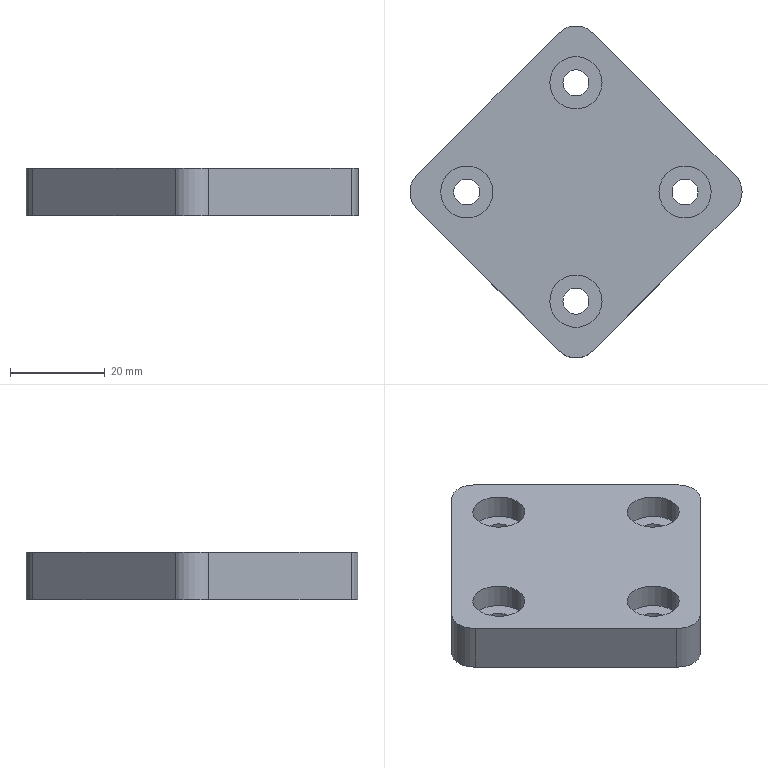Part | SolidWorks | features BaseBody 1 | 1 solid | 31 faces | box 70 x 70 x 10 mm | volume 24895 mm3 | cylinder 21 | plane 10 | commonest cylinder face diameters 5.5 x8 11 x8 10 x5
STEP:
#1=CARTESIAN_POINT('',(-699.595,684.746,545.732));
#2=VERTEX_POINT('',#1);
#3=CARTESIAN_POINT('',(-698.131,681.211,545.732));
#4=VERTEX_POINT('',#3);
#5=CARTESIAN_POINT('',(-703.131,681.211,545.732));
#6=DIRECTION('',(0.,0.,-1.));
#7=DIRECTION('',(0.7071,0.7071,0.));
#8=AXIS2_PLACEMENT_3D('',#5,#6,#7);
#9=CIRCLE('',#8,5.);
#10=EDGE_CURVE('',#2,#4,#9,.T.);
#11=ORIENTED_EDGE('',*,*,#10,.T.);
#12=CARTESIAN_POINT('',(-698.131,681.211,535.732));
#13=VERTEX_POINT('',#12);
#14=CARTESIAN_POINT('',(-698.131,681.211,558.768));
#15=DIRECTION('',(0.,0.,-1.));
#16=VECTOR('',#15,1000.);
#17=LINE('',#14,#16);
#18=EDGE_CURVE('',#4,#13,#17,.T.);
#19=ORIENTED_EDGE('',*,*,#18,.T.);
#20=CARTESIAN_POINT('',(-699.595,684.746,535.732));
#21=VERTEX_POINT('',#20);
#22=CARTESIAN_POINT('',(-703.131,681.211,535.732));
#23=DIRECTION('',(0.,0.,1.));
#24=DIRECTION('',(0.7071,-0.7071,0.));
#25=AXIS2_PLACEMENT_3D('',#22,#23,#24);
#26=CIRCLE('',#25,5.);
#27=EDGE_CURVE('',#13,#21,#26,.T.);
#28=ORIENTED_EDGE('',*,*,#27,.T.);
#29=CARTESIAN_POINT('',(-699.595,684.746,545.732));
#30=DIRECTION('',(0.,0.,-1.));
#31=VECTOR('',#30,1000.);
#32=LINE('',#29,#31);
#33=EDGE_CURVE('',#2,#21,#32,.T.);
#34=ORIENTED_EDGE('',*,*,#33,.F.);
#35=EDGE_LOOP('',(#11,#19,#28,#34));
#36=FACE_OUTER_BOUND('',#35,.T.);
#37=CARTESIAN_POINT('',(-703.131,681.211,558.768));
#38=DIRECTION('',(0.,0.,-1.));
#39=DIRECTION('',(1.,0.,0.));
#40=AXIS2_PLACEMENT_3D('',#37,#38,#39);
#41=CYLINDRICAL_SURFACE('',#40,5.);
#42=ADVANCED_FACE('',(#36),#41,.T.);
#43=CARTESIAN_POINT('',(-729.595,714.746,535.732));
#44=VERTEX_POINT('',#43);
#45=CARTESIAN_POINT('',(-736.666,714.746,535.732));
#46=VERTEX_POINT('',#45);
#47=CARTESIAN_POINT('',(-733.131,711.211,535.732));
#48=DIRECTION('',(0.,0.,1.));
#49=DIRECTION('',(0.7071,0.7071,0.));
#50=AXIS2_PLACEMENT_3D('',#47,#48,#49);
#51=CIRCLE('',#50,5.);
#52=EDGE_CURVE('',#44,#46,#51,.T.);
#53=ORIENTED_EDGE('',*,*,#52,.F.);
#54=CARTESIAN_POINT('',(-699.595,684.746,535.732));
#55=DIRECTION('',(-0.7071,0.7071,0.));
#56=VECTOR('',#55,1000.);
#57=LINE('',#54,#56);
#58=EDGE_CURVE('',#21,#44,#57,.T.);
#59=ORIENTED_EDGE('',*,*,#58,.F.);
#60=ORIENTED_EDGE('',*,*,#27,.F.);
#61=CARTESIAN_POINT('',(-699.595,677.675,535.732));
#62=VERTEX_POINT('',#61);
#63=CARTESIAN_POINT('',(-703.131,681.211,535.732));
#64=DIRECTION('',(0.,0.,1.));
#65=DIRECTION('',(0.7071,-0.7071,0.));
#66=AXIS2_PLACEMENT_3D('',#63,#64,#65);
#67=CIRCLE('',#66,5.);
#68=EDGE_CURVE('',#62,#13,#67,.T.);
#69=ORIENTED_EDGE('',*,*,#68,.F.);
#70=CARTESIAN_POINT('',(-729.595,647.675,535.732));
#71=VERTEX_POINT('',#70);
#72=CARTESIAN_POINT('',(-729.595,647.675,535.732));
#73=DIRECTION('',(0.7071,0.7071,0.));
#74=VECTOR('',#73,1000.);
#75=LINE('',#72,#74);
#76=EDGE_CURVE('',#71,#62,#75,.T.);
#77=ORIENTED_EDGE('',*,*,#76,.F.);
#78=CARTESIAN_POINT('',(-736.666,647.675,535.732));
#79=VERTEX_POINT('',#78);
#80=CARTESIAN_POINT('',(-733.131,651.211,535.732));
#81=DIRECTION('',(0.,0.,1.));
#82=DIRECTION('',(-0.7071,-0.7071,0.));
#83=AXIS2_PLACEMENT_3D('',#80,#81,#82);
#84=CIRCLE('',#83,5.);
#85=EDGE_CURVE('',#79,#71,#84,.T.);
#86=ORIENTED_EDGE('',*,*,#85,.F.);
#87=CARTESIAN_POINT('',(-766.666,677.675,535.732));
#88=VERTEX_POINT('',#87);
#89=CARTESIAN_POINT('',(-766.666,677.675,535.732));
#90=DIRECTION('',(0.7071,-0.7071,0.));
#91=VECTOR('',#90,1000.);
#92=LINE('',#89,#91);
#93=EDGE_CURVE('',#88,#79,#92,.T.);
#94=ORIENTED_EDGE('',*,*,#93,.F.);
#95=CARTESIAN_POINT('',(-766.666,684.746,535.732));
#96=VERTEX_POINT('',#95);
#97=CARTESIAN_POINT('',(-763.131,681.211,535.732));
#98=DIRECTION('',(0.,0.,1.));
#99=DIRECTION('',(-0.7071,0.7071,0.));
#100=AXIS2_PLACEMENT_3D('',#97,#98,#99);
#101=CIRCLE('',#100,5.);
#102=EDGE_CURVE('',#96,#88,#101,.T.);
#103=ORIENTED_EDGE('',*,*,#102,.F.);
#104=CARTESIAN_POINT('',(-736.666,714.746,535.732));
#105=DIRECTION('',(-0.7071,-0.7071,0.));
#106=VECTOR('',#105,1000.);
#107=LINE('',#104,#106);
#108=EDGE_CURVE('',#46,#96,#107,.T.);
#109=ORIENTED_EDGE('',*,*,#108,.F.);
#110=EDGE_LOOP('',(#53,#59,#60,#69,#77,#86,#94,#103,#109));
#111=FACE_OUTER_BOUND('',#110,.T.);
#112=CARTESIAN_POINT('',(-758.881,681.211,535.732));
#113=VERTEX_POINT('',#112);
#114=CARTESIAN_POINT('',(-753.381,681.211,535.732));
#115=VERTEX_POINT('',#114);
#116=CARTESIAN_POINT('',(-756.131,681.211,535.732));
#117=DIRECTION('',(0.,0.,-1.));
#118=DIRECTION('',(-1.,0.,0.));
#119=AXIS2_PLACEMENT_3D('',#116,#117,#118);
#120=CIRCLE('',#119,2.75);
#121=EDGE_CURVE('',#113,#115,#120,.T.);
#122=ORIENTED_EDGE('',*,*,#121,.F.);
#123=CARTESIAN_POINT('',(-756.131,681.211,535.732));
#124=DIRECTION('',(0.,0.,-1.));
#125=DIRECTION('',(1.,0.,0.));
#126=AXIS2_PLACEMENT_3D('',#123,#124,#125);
#127=CIRCLE('',#126,2.75);
#128=EDGE_CURVE('',#115,#113,#127,.T.);
#129=ORIENTED_EDGE('',*,*,#128,.F.);
#130=EDGE_LOOP('',(#122,#129));
#131=FACE_BOUND('',#130,.T.);
#132=CARTESIAN_POINT('',(-712.881,681.211,535.732));
#133=VERTEX_POINT('',#132);
#134=CARTESIAN_POINT('',(-707.381,681.211,535.732));
#135=VERTEX_POINT('',#134);
#136=CARTESIAN_POINT('',(-710.131,681.211,535.732));
#137=DIRECTION('',(0.,0.,-1.));
#138=DIRECTION('',(-1.,0.,0.));
#139=AXIS2_PLACEMENT_3D('',#136,#137,#138);
#140=CIRCLE('',#139,2.75);
#141=EDGE_CURVE('',#133,#135,#140,.T.);
#142=ORIENTED_EDGE('',*,*,#141,.F.);
#143=CARTESIAN_POINT('',(-710.131,681.211,535.732));
#144=DIRECTION('',(0.,0.,-1.));
#145=DIRECTION('',(1.,0.,0.));
#146=AXIS2_PLACEMENT_3D('',#143,#144,#145);
#147=CIRCLE('',#146,2.75);
#148=EDGE_CURVE('',#135,#133,#147,.T.);
#149=ORIENTED_EDGE('',*,*,#148,.F.);
#150=EDGE_LOOP('',(#142,#149));
#151=FACE_BOUND('',#150,.T.);
#152=CARTESIAN_POINT('',(-735.881,658.211,535.732));
#153=VERTEX_POINT('',#152);
#154=CARTESIAN_POINT('',(-730.381,658.211,535.732));
#155=VERTEX_POINT('',#154);
#156=CARTESIAN_POINT('',(-733.131,658.211,535.732));
#157=DIRECTION('',(0.,0.,-1.));
#158=DIRECTION('',(-1.,0.,0.));
#159=AXIS2_PLACEMENT_3D('',#156,#157,#158);
#160=CIRCLE('',#159,2.75);
#161=EDGE_CURVE('',#153,#155,#160,.T.);
#162=ORIENTED_EDGE('',*,*,#161,.F.);
#163=CARTESIAN_POINT('',(-733.131,658.211,535.732));
#164=DIRECTION('',(0.,0.,-1.));
#165=DIRECTION('',(1.,0.,0.));
#166=AXIS2_PLACEMENT_3D('',#163,#164,#165);
#167=CIRCLE('',#166,2.75);
#168=EDGE_CURVE('',#155,#153,#167,.T.);
#169=ORIENTED_EDGE('',*,*,#168,.F.);
#170=EDGE_LOOP('',(#162,#169));
#171=FACE_BOUND('',#170,.T.);
#172=CARTESIAN_POINT('',(-735.881,704.211,535.732));
#173=VERTEX_POINT('',#172);
#174=CARTESIAN_POINT('',(-730.381,704.211,535.732));
#175=VERTEX_POINT('',#174);
#176=CARTESIAN_POINT('',(-733.131,704.211,535.732));
#177=DIRECTION('',(0.,0.,-1.));
#178=DIRECTION('',(-1.,0.,0.));
#179=AXIS2_PLACEMENT_3D('',#176,#177,#178);
#180=CIRCLE('',#179,2.75);
#181=EDGE_CURVE('',#173,#175,#180,.T.);
#182=ORIENTED_EDGE('',*,*,#181,.F.);
#183=CARTESIAN_POINT('',(-733.131,704.211,535.732));
#184=DIRECTION('',(0.,0.,-1.));
#185=DIRECTION('',(1.,0.,0.));
#186=AXIS2_PLACEMENT_3D('',#183,#184,#185);
#187=CIRCLE('',#186,2.75);
#188=EDGE_CURVE('',#175,#173,#187,.T.);
#189=ORIENTED_EDGE('',*,*,#188,.F.);
#190=EDGE_LOOP('',(#182,#189));
#191=FACE_BOUND('',#190,.T.);
#192=CARTESIAN_POINT('',(0.,0.,535.732));
#193=DIRECTION('',(0.,0.,1.));
#194=DIRECTION('',(-1.,0.,0.));
#195=AXIS2_PLACEMENT_3D('',#192,#193,#194);
#196=PLANE('',#195);
#197=ADVANCED_FACE('',(#111,#131,#151,#171,#191),#196,.F.);
#198=CARTESIAN_POINT('',(-736.666,714.746,545.732));
#199=VERTEX_POINT('',#198);
#200=CARTESIAN_POINT('',(-736.666,714.746,545.732));
#201=DIRECTION('',(0.,0.,-1.));
#202=VECTOR('',#201,1000.);
#203=LINE('',#200,#202);
#204=EDGE_CURVE('',#199,#46,#203,.T.);
#205=ORIENTED_EDGE('',*,*,#204,.T.);
#206=ORIENTED_EDGE('',*,*,#108,.T.);
#207=CARTESIAN_POINT('',(-766.666,684.746,545.732));
#208=VERTEX_POINT('',#207);
#209=CARTESIAN_POINT('',(-766.666,684.746,535.732));
#210=DIRECTION('',(0.,0.,1.));
#211=VECTOR('',#210,1000.);
#212=LINE('',#209,#211);
#213=EDGE_CURVE('',#96,#208,#212,.T.);
#214=ORIENTED_EDGE('',*,*,#213,.T.);
#215=CARTESIAN_POINT('',(-766.666,684.746,545.732));
#216=DIRECTION('',(0.7071,0.7071,0.));
#217=VECTOR('',#216,1000.);
#218=LINE('',#215,#217);
#219=EDGE_CURVE('',#208,#199,#218,.T.);
#220=ORIENTED_EDGE('',*,*,#219,.T.);
#221=EDGE_LOOP('',(#205,#206,#214,#220));
#222=FACE_OUTER_BOUND('',#221,.T.);
#223=CARTESIAN_POINT('',(-733.131,718.282,535.732));
#224=DIRECTION('',(-0.7071,0.7071,0.));
#225=DIRECTION('',(0.7071,0.7071,0.));
#226=AXIS2_PLACEMENT_3D('',#223,#224,#225);
#227=PLANE('',#226);
#228=ADVANCED_FACE('',(#222),#227,.T.);
#229=CARTESIAN_POINT('',(-729.595,647.675,545.732));
#230=VERTEX_POINT('',#229);
#231=CARTESIAN_POINT('',(-736.666,647.675,545.732));
#232=VERTEX_POINT('',#231);
#233=CARTESIAN_POINT('',(-733.131,651.211,545.732));
#234=DIRECTION('',(0.,0.,-1.));
#235=DIRECTION('',(0.7071,-0.7071,0.));
#236=AXIS2_PLACEMENT_3D('',#233,#234,#235);
#237=CIRCLE('',#236,5.);
#238=EDGE_CURVE('',#230,#232,#237,.T.);
#239=ORIENTED_EDGE('',*,*,#238,.F.);
#240=CARTESIAN_POINT('',(-699.595,677.675,545.732));
#241=VERTEX_POINT('',#240);
#242=CARTESIAN_POINT('',(-699.595,677.675,545.732));
#243=DIRECTION('',(-0.7071,-0.7071,0.));
#244=VECTOR('',#243,1000.);
#245=LINE('',#242,#244);
#246=EDGE_CURVE('',#241,#230,#245,.T.);
#247=ORIENTED_EDGE('',*,*,#246,.F.);
#248=CARTESIAN_POINT('',(-703.131,681.211,545.732));
#249=DIRECTION('',(0.,0.,-1.));
#250=DIRECTION('',(0.7071,0.7071,0.));
#251=AXIS2_PLACEMENT_3D('',#248,#249,#250);
#252=CIRCLE('',#251,5.);
#253=EDGE_CURVE('',#4,#241,#252,.T.);
#254=ORIENTED_EDGE('',*,*,#253,.F.);
#255=ORIENTED_EDGE('',*,*,#10,.F.);
#256=CARTESIAN_POINT('',(-729.595,714.746,545.732));
#257=VERTEX_POINT('',#256);
#258=CARTESIAN_POINT('',(-729.595,714.746,545.732));
#259=DIRECTION('',(0.7071,-0.7071,0.));
#260=VECTOR('',#259,1000.);
#261=LINE('',#258,#260);
#262=EDGE_CURVE('',#257,#2,#261,.T.);
#263=ORIENTED_EDGE('',*,*,#262,.F.);
#264=CARTESIAN_POINT('',(-733.131,711.211,545.732));
#265=DIRECTION('',(0.,0.,-1.));
#266=DIRECTION('',(-0.7071,0.7071,0.));
#267=AXIS2_PLACEMENT_3D('',#264,#265,#266);
#268=CIRCLE('',#267,5.);
#269=EDGE_CURVE('',#199,#257,#268,.T.);
#270=ORIENTED_EDGE('',*,*,#269,.F.);
#271=ORIENTED_EDGE('',*,*,#219,.F.);
#272=CARTESIAN_POINT('',(-766.666,677.675,545.732));
#273=VERTEX_POINT('',#272);
#274=CARTESIAN_POINT('',(-763.131,681.211,545.732));
#275=DIRECTION('',(0.,0.,-1.));
#276=DIRECTION('',(-0.7071,-0.7071,0.));
#277=AXIS2_PLACEMENT_3D('',#274,#275,#276);
#278=CIRCLE('',#277,5.);
#279=EDGE_CURVE('',#273,#208,#278,.T.);
#280=ORIENTED_EDGE('',*,*,#279,.F.);
#281=CARTESIAN_POINT('',(-736.666,647.675,545.732));
#282=DIRECTION('',(-0.7071,0.7071,0.));
#283=VECTOR('',#282,1000.);
#284=LINE('',#281,#283);
#285=EDGE_CURVE('',#232,#273,#284,.T.);
#286=ORIENTED_EDGE('',*,*,#285,.F.);
#287=EDGE_LOOP('',(#239,#247,#254,#255,#263,#270,#271,#280,#286));
#288=FACE_OUTER_BOUND('',#287,.T.);
#289=CARTESIAN_POINT('',(-727.631,704.211,545.732));
#290=VERTEX_POINT('',#289);
#291=CARTESIAN_POINT('',(-738.631,704.211,545.732));
#292=VERTEX_POINT('',#291);
#293=CARTESIAN_POINT('',(-733.131,704.211,545.732));
#294=DIRECTION('',(0.,0.,1.));
#295=DIRECTION('',(1.,0.,0.));
#296=AXIS2_PLACEMENT_3D('',#293,#294,#295);
#297=CIRCLE('',#296,5.5);
#298=EDGE_CURVE('',#290,#292,#297,.T.);
#299=ORIENTED_EDGE('',*,*,#298,.F.);
#300=CARTESIAN_POINT('',(-733.131,704.211,545.732));
#301=DIRECTION('',(0.,0.,1.));
#302=DIRECTION('',(-1.,0.,0.));
#303=AXIS2_PLACEMENT_3D('',#300,#301,#302);
#304=CIRCLE('',#303,5.5);
#305=EDGE_CURVE('',#292,#290,#304,.T.);
#306=ORIENTED_EDGE('',*,*,#305,.F.);
#307=EDGE_LOOP('',(#299,#306));
#308=FACE_BOUND('',#307,.T.);
#309=CARTESIAN_POINT('',(-704.631,681.211,545.732));
#310=VERTEX_POINT('',#309);
#311=CARTESIAN_POINT('',(-715.631,681.211,545.732));
#312=VERTEX_POINT('',#311);
#313=CARTESIAN_POINT('',(-710.131,681.211,545.732));
#314=DIRECTION('',(0.,0.,1.));
#315=DIRECTION('',(1.,0.,0.));
#316=AXIS2_PLACEMENT_3D('',#313,#314,#315);
#317=CIRCLE('',#316,5.5);
#318=EDGE_CURVE('',#310,#312,#317,.T.);
#319=ORIENTED_EDGE('',*,*,#318,.F.);
#320=CARTESIAN_POINT('',(-710.131,681.211,545.732));
#321=DIRECTION('',(0.,0.,1.));
#322=DIRECTION('',(-1.,0.,0.));
#323=AXIS2_PLACEMENT_3D('',#320,#321,#322);
#324=CIRCLE('',#323,5.5);
#325=EDGE_CURVE('',#312,#310,#324,.T.);
#326=ORIENTED_EDGE('',*,*,#325,.F.);
#327=EDGE_LOOP('',(#319,#326));
#328=FACE_BOUND('',#327,.T.);
#329=CARTESIAN_POINT('',(-727.631,658.211,545.732));
#330=VERTEX_POINT('',#329);
#331=CARTESIAN_POINT('',(-738.631,658.211,545.732));
#332=VERTEX_POINT('',#331);
#333=CARTESIAN_POINT('',(-733.131,658.211,545.732));
#334=DIRECTION('',(0.,0.,1.));
#335=DIRECTION('',(1.,0.,0.));
#336=AXIS2_PLACEMENT_3D('',#333,#334,#335);
#337=CIRCLE('',#336,5.5);
#338=EDGE_CURVE('',#330,#332,#337,.T.);
#339=ORIENTED_EDGE('',*,*,#338,.F.);
#340=CARTESIAN_POINT('',(-733.131,658.211,545.732));
#341=DIRECTION('',(0.,0.,1.));
#342=DIRECTION('',(-1.,0.,0.));
#343=AXIS2_PLACEMENT_3D('',#340,#341,#342);
#344=CIRCLE('',#343,5.5);
#345=EDGE_CURVE('',#332,#330,#344,.T.);
#346=ORIENTED_EDGE('',*,*,#345,.F.);
#347=EDGE_LOOP('',(#339,#346));
#348=FACE_BOUND('',#347,.T.);
#349=CARTESIAN_POINT('',(-750.631,681.211,545.732));
#350=VERTEX_POINT('',#349);
#351=CARTESIAN_POINT('',(-761.631,681.211,545.732));
#352=VERTEX_POINT('',#351);
#353=CARTESIAN_POINT('',(-756.131,681.211,545.732));
#354=DIRECTION('',(0.,0.,1.));
#355=DIRECTION('',(1.,0.,0.));
#356=AXIS2_PLACEMENT_3D('',#353,#354,#355);
#357=CIRCLE('',#356,5.5);
#358=EDGE_CURVE('',#350,#352,#357,.T.);
#359=ORIENTED_EDGE('',*,*,#358,.F.);
#360=CARTESIAN_POINT('',(-756.131,681.211,545.732));
#361=DIRECTION('',(0.,0.,1.));
#362=DIRECTION('',(-1.,0.,0.));
#363=AXIS2_PLACEMENT_3D('',#360,#361,#362);
#364=CIRCLE('',#363,5.5);
#365=EDGE_CURVE('',#352,#350,#364,.T.);
#366=ORIENTED_EDGE('',*,*,#365,.F.);
#367=EDGE_LOOP('',(#359,#366));
#368=FACE_BOUND('',#367,.T.);
#369=CARTESIAN_POINT('',(0.,0.,545.732));
#370=DIRECTION('',(0.,0.,1.));
#371=DIRECTION('',(-1.,0.,0.));
#372=AXIS2_PLACEMENT_3D('',#369,#370,#371);
#373=PLANE('',#372);
#374=ADVANCED_FACE('',(#288,#308,#328,#348,#368),#373,.T.);
#375=CARTESIAN_POINT('',(-736.666,647.675,535.732));
#376=DIRECTION('',(0.,0.,1.));
#377=VECTOR('',#376,1000.);
#378=LINE('',#375,#377);
#379=EDGE_CURVE('',#79,#232,#378,.T.);
#380=ORIENTED_EDGE('',*,*,#379,.T.);
#381=ORIENTED_EDGE('',*,*,#285,.T.);
#382=CARTESIAN_POINT('',(-766.666,677.675,545.732));
#383=DIRECTION('',(0.,0.,-1.));
#384=VECTOR('',#383,1000.);
#385=LINE('',#382,#384);
#386=EDGE_CURVE('',#273,#88,#385,.T.);
#387=ORIENTED_EDGE('',*,*,#386,.T.);
#388=ORIENTED_EDGE('',*,*,#93,.T.);
#389=EDGE_LOOP('',(#380,#381,#387,#388));
#390=FACE_OUTER_BOUND('',#389,.T.);
#391=CARTESIAN_POINT('',(-770.202,681.211,535.732));
#392=DIRECTION('',(-0.7071,-0.7071,0.));
#393=DIRECTION('',(-0.7071,0.7071,0.));
#394=AXIS2_PLACEMENT_3D('',#391,#392,#393);
#395=PLANE('',#394);
#396=ADVANCED_FACE('',(#390),#395,.T.);
#397=ORIENTED_EDGE('',*,*,#279,.T.);
#398=ORIENTED_EDGE('',*,*,#213,.F.);
#399=ORIENTED_EDGE('',*,*,#102,.T.);
#400=ORIENTED_EDGE('',*,*,#386,.F.);
#401=EDGE_LOOP('',(#397,#398,#399,#400));
#402=FACE_OUTER_BOUND('',#401,.T.);
#403=CARTESIAN_POINT('',(-763.131,681.211,558.768));
#404=DIRECTION('',(0.,0.,-1.));
#405=DIRECTION('',(1.,0.,0.));
#406=AXIS2_PLACEMENT_3D('',#403,#404,#405);
#407=CYLINDRICAL_SURFACE('',#406,5.);
#408=ADVANCED_FACE('',(#402),#407,.T.);
#409=ORIENTED_EDGE('',*,*,#238,.T.);
#410=ORIENTED_EDGE('',*,*,#379,.F.);
#411=ORIENTED_EDGE('',*,*,#85,.T.);
#412=CARTESIAN_POINT('',(-729.595,647.675,545.732));
#413=DIRECTION('',(0.,0.,-1.));
#414=VECTOR('',#413,1000.);
#415=LINE('',#412,#414);
#416=EDGE_CURVE('',#230,#71,#415,.T.);
#417=ORIENTED_EDGE('',*,*,#416,.F.);
#418=EDGE_LOOP('',(#409,#410,#411,#417));
#419=FACE_OUTER_BOUND('',#418,.T.);
#420=CARTESIAN_POINT('',(-733.131,651.211,558.768));
#421=DIRECTION('',(0.,0.,-1.));
#422=DIRECTION('',(1.,0.,0.));
#423=AXIS2_PLACEMENT_3D('',#420,#421,#422);
#424=CYLINDRICAL_SURFACE('',#423,5.);
#425=ADVANCED_FACE('',(#419),#424,.T.);
#426=CARTESIAN_POINT('',(-699.595,677.675,535.732));
#427=DIRECTION('',(0.,0.,1.));
#428=VECTOR('',#427,1000.);
#429=LINE('',#426,#428);
#430=EDGE_CURVE('',#62,#241,#429,.T.);
#431=ORIENTED_EDGE('',*,*,#430,.T.);
#432=ORIENTED_EDGE('',*,*,#246,.T.);
#433=ORIENTED_EDGE('',*,*,#416,.T.);
#434=ORIENTED_EDGE('',*,*,#76,.T.);
#435=EDGE_LOOP('',(#431,#432,#433,#434));
#436=FACE_OUTER_BOUND('',#435,.T.);
#437=CARTESIAN_POINT('',(-733.131,644.139,535.732));
#438=DIRECTION('',(0.7071,-0.7071,0.));
#439=DIRECTION('',(-0.7071,-0.7071,0.));
#440=AXIS2_PLACEMENT_3D('',#437,#438,#439);
#441=PLANE('',#440);
#442=ADVANCED_FACE('',(#436),#441,.T.);
#443=ORIENTED_EDGE('',*,*,#18,.F.);
#444=ORIENTED_EDGE('',*,*,#253,.T.);
#445=ORIENTED_EDGE('',*,*,#430,.F.);
#446=ORIENTED_EDGE('',*,*,#68,.T.);
#447=EDGE_LOOP('',(#443,#444,#445,#446));
#448=FACE_OUTER_BOUND('',#447,.T.);
#449=CARTESIAN_POINT('',(-703.131,681.211,558.768));
#450=DIRECTION('',(0.,0.,-1.));
#451=DIRECTION('',(1.,0.,0.));
#452=AXIS2_PLACEMENT_3D('',#449,#450,#451);
#453=CYLINDRICAL_SURFACE('',#452,5.);
#454=ADVANCED_FACE('',(#448),#453,.T.);
#455=ORIENTED_EDGE('',*,*,#33,.T.);
#456=ORIENTED_EDGE('',*,*,#58,.T.);
#457=CARTESIAN_POINT('',(-729.595,714.746,535.732));
#458=DIRECTION('',(0.,0.,1.));
#459=VECTOR('',#458,1000.);
#460=LINE('',#457,#459);
#461=EDGE_CURVE('',#44,#257,#460,.T.);
#462=ORIENTED_EDGE('',*,*,#461,.T.);
#463=ORIENTED_EDGE('',*,*,#262,.T.);
#464=EDGE_LOOP('',(#455,#456,#462,#463));
#465=FACE_OUTER_BOUND('',#464,.T.);
#466=CARTESIAN_POINT('',(-696.06,681.211,535.732));
#467=DIRECTION('',(0.7071,0.7071,0.));
#468=DIRECTION('',(0.7071,-0.7071,0.));
#469=AXIS2_PLACEMENT_3D('',#466,#467,#468);
#470=PLANE('',#469);
#471=ADVANCED_FACE('',(#465),#470,.T.);
#472=ORIENTED_EDGE('',*,*,#269,.T.);
#473=ORIENTED_EDGE('',*,*,#461,.F.);
#474=ORIENTED_EDGE('',*,*,#52,.T.);
#475=ORIENTED_EDGE('',*,*,#204,.F.);
#476=EDGE_LOOP('',(#472,#473,#474,#475));
#477=FACE_OUTER_BOUND('',#476,.T.);
#478=CARTESIAN_POINT('',(-733.131,711.211,558.768));
#479=DIRECTION('',(0.,0.,-1.));
#480=DIRECTION('',(1.,0.,0.));
#481=AXIS2_PLACEMENT_3D('',#478,#479,#480);
#482=CYLINDRICAL_SURFACE('',#481,5.);
#483=ADVANCED_FACE('',(#477),#482,.T.);
#484=CARTESIAN_POINT('',(-727.631,704.211,540.732));
#485=VERTEX_POINT('',#484);
#486=CARTESIAN_POINT('',(-738.631,704.211,540.732));
#487=VERTEX_POINT('',#486);
#488=CARTESIAN_POINT('',(-733.131,704.211,540.732));
#489=DIRECTION('',(0.,0.,-1.));
#490=DIRECTION('',(1.,0.,0.));
#491=AXIS2_PLACEMENT_3D('',#488,#489,#490);
#492=CIRCLE('',#491,5.5);
#493=EDGE_CURVE('',#485,#487,#492,.T.);
#494=ORIENTED_EDGE('',*,*,#493,.T.);
#495=CARTESIAN_POINT('',(-738.631,704.211,540.732));
#496=DIRECTION('',(0.,0.,1.));
#497=VECTOR('',#496,1000.);
#498=LINE('',#495,#497);
#499=EDGE_CURVE('',#487,#292,#498,.T.);
#500=ORIENTED_EDGE('',*,*,#499,.T.);
#501=ORIENTED_EDGE('',*,*,#305,.T.);
#502=CARTESIAN_POINT('',(-727.631,704.211,545.732));
#503=DIRECTION('',(0.,0.,-1.));
#504=VECTOR('',#503,1000.);
#505=LINE('',#502,#504);
#506=EDGE_CURVE('',#290,#485,#505,.T.);
#507=ORIENTED_EDGE('',*,*,#506,.T.);
#508=EDGE_LOOP('',(#494,#500,#501,#507));
#509=FACE_OUTER_BOUND('',#508,.T.);
#510=CARTESIAN_POINT('',(-733.131,704.211,545.732));
#511=DIRECTION('',(0.,0.,1.));
#512=DIRECTION('',(-1.,0.,0.));
#513=AXIS2_PLACEMENT_3D('',#510,#511,#512);
#514=CYLINDRICAL_SURFACE('',#513,5.5);
#515=ADVANCED_FACE('',(#509),#514,.F.);
#516=CARTESIAN_POINT('',(-733.131,704.211,540.732));
#517=DIRECTION('',(0.,0.,-1.));
#518=DIRECTION('',(-1.,0.,0.));
#519=AXIS2_PLACEMENT_3D('',#516,#517,#518);
#520=CIRCLE('',#519,5.5);
#521=EDGE_CURVE('',#487,#485,#520,.T.);
#522=ORIENTED_EDGE('',*,*,#521,.T.);
#523=ORIENTED_EDGE('',*,*,#506,.F.);
#524=ORIENTED_EDGE('',*,*,#298,.T.);
#525=ORIENTED_EDGE('',*,*,#499,.F.);
#526=EDGE_LOOP('',(#522,#523,#524,#525));
#527=FACE_OUTER_BOUND('',#526,.T.);
#528=CARTESIAN_POINT('',(-733.131,704.211,545.732));
#529=DIRECTION('',(0.,0.,1.));
#530=DIRECTION('',(-1.,0.,0.));
#531=AXIS2_PLACEMENT_3D('',#528,#529,#530);
#532=CYLINDRICAL_SURFACE('',#531,5.5);
#533=ADVANCED_FACE('',(#527),#532,.F.);
#534=ORIENTED_EDGE('',*,*,#521,.F.);
#535=ORIENTED_EDGE('',*,*,#493,.F.);
#536=EDGE_LOOP('',(#534,#535));
#537=FACE_OUTER_BOUND('',#536,.T.);
#538=CARTESIAN_POINT('',(-730.381,704.211,540.732));
#539=VERTEX_POINT('',#538);
#540=CARTESIAN_POINT('',(-735.881,704.211,540.732));
#541=VERTEX_POINT('',#540);
#542=CARTESIAN_POINT('',(-733.131,704.211,540.732));
#543=DIRECTION('',(0.,0.,1.));
#544=DIRECTION('',(1.,0.,0.));
#545=AXIS2_PLACEMENT_3D('',#542,#543,#544);
#546=CIRCLE('',#545,2.75);
#547=EDGE_CURVE('',#539,#541,#546,.T.);
#548=ORIENTED_EDGE('',*,*,#547,.F.);
#549=CARTESIAN_POINT('',(-733.131,704.211,540.732));
#550=DIRECTION('',(0.,0.,1.));
#551=DIRECTION('',(-1.,0.,0.));
#552=AXIS2_PLACEMENT_3D('',#549,#550,#551);
#553=CIRCLE('',#552,2.75);
#554=EDGE_CURVE('',#541,#539,#553,.T.);
#555=ORIENTED_EDGE('',*,*,#554,.F.);
#556=EDGE_LOOP('',(#548,#555));
#557=FACE_BOUND('',#556,.T.);
#558=CARTESIAN_POINT('',(0.,0.,540.732));
#559=DIRECTION('',(0.,0.,1.));
#560=DIRECTION('',(-1.,0.,0.));
#561=AXIS2_PLACEMENT_3D('',#558,#559,#560);
#562=PLANE('',#561);
#563=ADVANCED_FACE('',(#537,#557),#562,.T.);
#564=ORIENTED_EDGE('',*,*,#188,.T.);
#565=CARTESIAN_POINT('',(-735.881,704.211,535.732));
#566=DIRECTION('',(0.,0.,1.));
#567=VECTOR('',#566,1000.);
#568=LINE('',#565,#567);
#569=EDGE_CURVE('',#173,#541,#568,.T.);
#570=ORIENTED_EDGE('',*,*,#569,.T.);
#571=ORIENTED_EDGE('',*,*,#554,.T.);
#572=CARTESIAN_POINT('',(-730.381,704.211,540.732));
#573=DIRECTION('',(0.,0.,-1.));
#574=VECTOR('',#573,1000.);
#575=LINE('',#572,#574);
#576=EDGE_CURVE('',#539,#175,#575,.T.);
#577=ORIENTED_EDGE('',*,*,#576,.T.);
#578=EDGE_LOOP('',(#564,#570,#571,#577));
#579=FACE_OUTER_BOUND('',#578,.T.);
#580=CARTESIAN_POINT('',(-733.131,704.211,545.732));
#581=DIRECTION('',(0.,0.,1.));
#582=DIRECTION('',(-1.,0.,0.));
#583=AXIS2_PLACEMENT_3D('',#580,#581,#582);
#584=CYLINDRICAL_SURFACE('',#583,2.75);
#585=ADVANCED_FACE('',(#579),#584,.F.);
#586=ORIENTED_EDGE('',*,*,#181,.T.);
#587=ORIENTED_EDGE('',*,*,#576,.F.);
#588=ORIENTED_EDGE('',*,*,#547,.T.);
#589=ORIENTED_EDGE('',*,*,#569,.F.);
#590=EDGE_LOOP('',(#586,#587,#588,#589));
#591=FACE_OUTER_BOUND('',#590,.T.);
#592=CARTESIAN_POINT('',(-733.131,704.211,545.732));
#593=DIRECTION('',(0.,0.,1.));
#594=DIRECTION('',(-1.,0.,0.));
#595=AXIS2_PLACEMENT_3D('',#592,#593,#594);
#596=CYLINDRICAL_SURFACE('',#595,2.75);
#597=ADVANCED_FACE('',(#591),#596,.F.);
#598=CARTESIAN_POINT('',(-704.631,681.211,540.732));
#599=VERTEX_POINT('',#598);
#600=CARTESIAN_POINT('',(-715.631,681.211,540.732));
#601=VERTEX_POINT('',#600);
#602=CARTESIAN_POINT('',(-710.131,681.211,540.732));
#603=DIRECTION('',(0.,0.,-1.));
#604=DIRECTION('',(1.,0.,0.));
#605=AXIS2_PLACEMENT_3D('',#602,#603,#604);
#606=CIRCLE('',#605,5.5);
#607=EDGE_CURVE('',#599,#601,#606,.T.);
#608=ORIENTED_EDGE('',*,*,#607,.T.);
#609=CARTESIAN_POINT('',(-715.631,681.211,540.732));
#610=DIRECTION('',(0.,0.,1.));
#611=VECTOR('',#610,1000.);
#612=LINE('',#609,#611);
#613=EDGE_CURVE('',#601,#312,#612,.T.);
#614=ORIENTED_EDGE('',*,*,#613,.T.);
#615=ORIENTED_EDGE('',*,*,#325,.T.);
#616=CARTESIAN_POINT('',(-704.631,681.211,545.732));
#617=DIRECTION('',(0.,0.,-1.));
#618=VECTOR('',#617,1000.);
#619=LINE('',#616,#618);
#620=EDGE_CURVE('',#310,#599,#619,.T.);
#621=ORIENTED_EDGE('',*,*,#620,.T.);
#622=EDGE_LOOP('',(#608,#614,#615,#621));
#623=FACE_OUTER_BOUND('',#622,.T.);
#624=CARTESIAN_POINT('',(-710.131,681.211,545.732));
#625=DIRECTION('',(0.,0.,1.));
#626=DIRECTION('',(-1.,0.,0.));
#627=AXIS2_PLACEMENT_3D('',#624,#625,#626);
#628=CYLINDRICAL_SURFACE('',#627,5.5);
#629=ADVANCED_FACE('',(#623),#628,.F.);
#630=CARTESIAN_POINT('',(-710.131,681.211,540.732));
#631=DIRECTION('',(0.,0.,-1.));
#632=DIRECTION('',(-1.,0.,0.));
#633=AXIS2_PLACEMENT_3D('',#630,#631,#632);
#634=CIRCLE('',#633,5.5);
#635=EDGE_CURVE('',#601,#599,#634,.T.);
#636=ORIENTED_EDGE('',*,*,#635,.T.);
#637=ORIENTED_EDGE('',*,*,#620,.F.);
#638=ORIENTED_EDGE('',*,*,#318,.T.);
#639=ORIENTED_EDGE('',*,*,#613,.F.);
#640=EDGE_LOOP('',(#636,#637,#638,#639));
#641=FACE_OUTER_BOUND('',#640,.T.);
#642=CARTESIAN_POINT('',(-710.131,681.211,545.732));
#643=DIRECTION('',(0.,0.,1.));
#644=DIRECTION('',(-1.,0.,0.));
#645=AXIS2_PLACEMENT_3D('',#642,#643,#644);
#646=CYLINDRICAL_SURFACE('',#645,5.5);
#647=ADVANCED_FACE('',(#641),#646,.F.);
#648=ORIENTED_EDGE('',*,*,#635,.F.);
#649=ORIENTED_EDGE('',*,*,#607,.F.);
#650=EDGE_LOOP('',(#648,#649));
#651=FACE_OUTER_BOUND('',#650,.T.);
#652=CARTESIAN_POINT('',(-707.381,681.211,540.732));
#653=VERTEX_POINT('',#652);
#654=CARTESIAN_POINT('',(-712.881,681.211,540.732));
#655=VERTEX_POINT('',#654);
#656=CARTESIAN_POINT('',(-710.131,681.211,540.732));
#657=DIRECTION('',(0.,0.,1.));
#658=DIRECTION('',(1.,0.,0.));
#659=AXIS2_PLACEMENT_3D('',#656,#657,#658);
#660=CIRCLE('',#659,2.75);
#661=EDGE_CURVE('',#653,#655,#660,.T.);
#662=ORIENTED_EDGE('',*,*,#661,.F.);
#663=CARTESIAN_POINT('',(-710.131,681.211,540.732));
#664=DIRECTION('',(0.,0.,1.));
#665=DIRECTION('',(-1.,0.,0.));
#666=AXIS2_PLACEMENT_3D('',#663,#664,#665);
#667=CIRCLE('',#666,2.75);
#668=EDGE_CURVE('',#655,#653,#667,.T.);
#669=ORIENTED_EDGE('',*,*,#668,.F.);
#670=EDGE_LOOP('',(#662,#669));
#671=FACE_BOUND('',#670,.T.);
#672=CARTESIAN_POINT('',(0.,0.,540.732));
#673=DIRECTION('',(0.,0.,1.));
#674=DIRECTION('',(-1.,0.,0.));
#675=AXIS2_PLACEMENT_3D('',#672,#673,#674);
#676=PLANE('',#675);
#677=ADVANCED_FACE('',(#651,#671),#676,.T.);
#678=ORIENTED_EDGE('',*,*,#148,.T.);
#679=CARTESIAN_POINT('',(-712.881,681.211,535.732));
#680=DIRECTION('',(0.,0.,1.));
#681=VECTOR('',#680,1000.);
#682=LINE('',#679,#681);
#683=EDGE_CURVE('',#133,#655,#682,.T.);
#684=ORIENTED_EDGE('',*,*,#683,.T.);
#685=ORIENTED_EDGE('',*,*,#668,.T.);
#686=CARTESIAN_POINT('',(-707.381,681.211,540.732));
#687=DIRECTION('',(0.,0.,-1.));
#688=VECTOR('',#687,1000.);
#689=LINE('',#686,#688);
#690=EDGE_CURVE('',#653,#135,#689,.T.);
#691=ORIENTED_EDGE('',*,*,#690,.T.);
#692=EDGE_LOOP('',(#678,#684,#685,#691));
#693=FACE_OUTER_BOUND('',#692,.T.);
#694=CARTESIAN_POINT('',(-710.131,681.211,545.732));
#695=DIRECTION('',(0.,0.,1.));
#696=DIRECTION('',(-1.,0.,0.));
#697=AXIS2_PLACEMENT_3D('',#694,#695,#696);
#698=CYLINDRICAL_SURFACE('',#697,2.75);
#699=ADVANCED_FACE('',(#693),#698,.F.);
#700=ORIENTED_EDGE('',*,*,#141,.T.);
#701=ORIENTED_EDGE('',*,*,#690,.F.);
#702=ORIENTED_EDGE('',*,*,#661,.T.);
#703=ORIENTED_EDGE('',*,*,#683,.F.);
#704=EDGE_LOOP('',(#700,#701,#702,#703));
#705=FACE_OUTER_BOUND('',#704,.T.);
#706=CARTESIAN_POINT('',(-710.131,681.211,545.732));
#707=DIRECTION('',(0.,0.,1.));
#708=DIRECTION('',(-1.,0.,0.));
#709=AXIS2_PLACEMENT_3D('',#706,#707,#708);
#710=CYLINDRICAL_SURFACE('',#709,2.75);
#711=ADVANCED_FACE('',(#705),#710,.F.);
#712=CARTESIAN_POINT('',(-727.631,658.211,540.732));
#713=VERTEX_POINT('',#712);
#714=CARTESIAN_POINT('',(-738.631,658.211,540.732));
#715=VERTEX_POINT('',#714);
#716=CARTESIAN_POINT('',(-733.131,658.211,540.732));
#717=DIRECTION('',(0.,0.,-1.));
#718=DIRECTION('',(1.,0.,0.));
#719=AXIS2_PLACEMENT_3D('',#716,#717,#718);
#720=CIRCLE('',#719,5.5);
#721=EDGE_CURVE('',#713,#715,#720,.T.);
#722=ORIENTED_EDGE('',*,*,#721,.T.);
#723=CARTESIAN_POINT('',(-738.631,658.211,540.732));
#724=DIRECTION('',(0.,0.,1.));
#725=VECTOR('',#724,1000.);
#726=LINE('',#723,#725);
#727=EDGE_CURVE('',#715,#332,#726,.T.);
#728=ORIENTED_EDGE('',*,*,#727,.T.);
#729=ORIENTED_EDGE('',*,*,#345,.T.);
#730=CARTESIAN_POINT('',(-727.631,658.211,545.732));
#731=DIRECTION('',(0.,0.,-1.));
#732=VECTOR('',#731,1000.);
#733=LINE('',#730,#732);
#734=EDGE_CURVE('',#330,#713,#733,.T.);
#735=ORIENTED_EDGE('',*,*,#734,.T.);
#736=EDGE_LOOP('',(#722,#728,#729,#735));
#737=FACE_OUTER_BOUND('',#736,.T.);
#738=CARTESIAN_POINT('',(-733.131,658.211,545.732));
#739=DIRECTION('',(0.,0.,1.));
#740=DIRECTION('',(-1.,0.,0.));
#741=AXIS2_PLACEMENT_3D('',#738,#739,#740);
#742=CYLINDRICAL_SURFACE('',#741,5.5);
#743=ADVANCED_FACE('',(#737),#742,.F.);
#744=CARTESIAN_POINT('',(-733.131,658.211,540.732));
#745=DIRECTION('',(0.,0.,-1.));
#746=DIRECTION('',(-1.,0.,0.));
#747=AXIS2_PLACEMENT_3D('',#744,#745,#746);
#748=CIRCLE('',#747,5.5);
#749=EDGE_CURVE('',#715,#713,#748,.T.);
#750=ORIENTED_EDGE('',*,*,#749,.T.);
#751=ORIENTED_EDGE('',*,*,#734,.F.);
#752=ORIENTED_EDGE('',*,*,#338,.T.);
#753=ORIENTED_EDGE('',*,*,#727,.F.);
#754=EDGE_LOOP('',(#750,#751,#752,#753));
#755=FACE_OUTER_BOUND('',#754,.T.);
#756=CARTESIAN_POINT('',(-733.131,658.211,545.732));
#757=DIRECTION('',(0.,0.,1.));
#758=DIRECTION('',(-1.,0.,0.));
#759=AXIS2_PLACEMENT_3D('',#756,#757,#758);
#760=CYLINDRICAL_SURFACE('',#759,5.5);
#761=ADVANCED_FACE('',(#755),#760,.F.);
#762=ORIENTED_EDGE('',*,*,#749,.F.);
#763=ORIENTED_EDGE('',*,*,#721,.F.);
#764=EDGE_LOOP('',(#762,#763));
#765=FACE_OUTER_BOUND('',#764,.T.);
#766=CARTESIAN_POINT('',(-730.381,658.211,540.732));
#767=VERTEX_POINT('',#766);
#768=CARTESIAN_POINT('',(-735.881,658.211,540.732));
#769=VERTEX_POINT('',#768);
#770=CARTESIAN_POINT('',(-733.131,658.211,540.732));
#771=DIRECTION('',(0.,0.,1.));
#772=DIRECTION('',(1.,0.,0.));
#773=AXIS2_PLACEMENT_3D('',#770,#771,#772);
#774=CIRCLE('',#773,2.75);
#775=EDGE_CURVE('',#767,#769,#774,.T.);
#776=ORIENTED_EDGE('',*,*,#775,.F.);
#777=CARTESIAN_POINT('',(-733.131,658.211,540.732));
#778=DIRECTION('',(0.,0.,1.));
#779=DIRECTION('',(-1.,0.,0.));
#780=AXIS2_PLACEMENT_3D('',#777,#778,#779);
#781=CIRCLE('',#780,2.75);
#782=EDGE_CURVE('',#769,#767,#781,.T.);
#783=ORIENTED_EDGE('',*,*,#782,.F.);
#784=EDGE_LOOP('',(#776,#783));
#785=FACE_BOUND('',#784,.T.);
#786=CARTESIAN_POINT('',(0.,0.,540.732));
#787=DIRECTION('',(0.,0.,1.));
#788=DIRECTION('',(-1.,0.,0.));
#789=AXIS2_PLACEMENT_3D('',#786,#787,#788);
#790=PLANE('',#789);
#791=ADVANCED_FACE('',(#765,#785),#790,.T.);
#792=ORIENTED_EDGE('',*,*,#168,.T.);
#793=CARTESIAN_POINT('',(-735.881,658.211,535.732));
#794=DIRECTION('',(0.,0.,1.));
#795=VECTOR('',#794,1000.);
#796=LINE('',#793,#795);
#797=EDGE_CURVE('',#153,#769,#796,.T.);
#798=ORIENTED_EDGE('',*,*,#797,.T.);
#799=ORIENTED_EDGE('',*,*,#782,.T.);
#800=CARTESIAN_POINT('',(-730.381,658.211,540.732));
#801=DIRECTION('',(0.,0.,-1.));
#802=VECTOR('',#801,1000.);
#803=LINE('',#800,#802);
#804=EDGE_CURVE('',#767,#155,#803,.T.);
#805=ORIENTED_EDGE('',*,*,#804,.T.);
#806=EDGE_LOOP('',(#792,#798,#799,#805));
#807=FACE_OUTER_BOUND('',#806,.T.);
#808=CARTESIAN_POINT('',(-733.131,658.211,545.732));
#809=DIRECTION('',(0.,0.,1.));
#810=DIRECTION('',(-1.,0.,0.));
#811=AXIS2_PLACEMENT_3D('',#808,#809,#810);
#812=CYLINDRICAL_SURFACE('',#811,2.75);
#813=ADVANCED_FACE('',(#807),#812,.F.);
#814=ORIENTED_EDGE('',*,*,#161,.T.);
#815=ORIENTED_EDGE('',*,*,#804,.F.);
#816=ORIENTED_EDGE('',*,*,#775,.T.);
#817=ORIENTED_EDGE('',*,*,#797,.F.);
#818=EDGE_LOOP('',(#814,#815,#816,#817));
#819=FACE_OUTER_BOUND('',#818,.T.);
#820=CARTESIAN_POINT('',(-733.131,658.211,545.732));
#821=DIRECTION('',(0.,0.,1.));
#822=DIRECTION('',(-1.,0.,0.));
#823=AXIS2_PLACEMENT_3D('',#820,#821,#822);
#824=CYLINDRICAL_SURFACE('',#823,2.75);
#825=ADVANCED_FACE('',(#819),#824,.F.);
#826=CARTESIAN_POINT('',(-750.631,681.211,540.732));
#827=VERTEX_POINT('',#826);
#828=CARTESIAN_POINT('',(-761.631,681.211,540.732));
#829=VERTEX_POINT('',#828);
#830=CARTESIAN_POINT('',(-756.131,681.211,540.732));
#831=DIRECTION('',(0.,0.,-1.));
#832=DIRECTION('',(1.,0.,0.));
#833=AXIS2_PLACEMENT_3D('',#830,#831,#832);
#834=CIRCLE('',#833,5.5);
#835=EDGE_CURVE('',#827,#829,#834,.T.);
#836=ORIENTED_EDGE('',*,*,#835,.T.);
#837=CARTESIAN_POINT('',(-761.631,681.211,540.732));
#838=DIRECTION('',(0.,0.,1.));
#839=VECTOR('',#838,1000.);
#840=LINE('',#837,#839);
#841=EDGE_CURVE('',#829,#352,#840,.T.);
#842=ORIENTED_EDGE('',*,*,#841,.T.);
#843=ORIENTED_EDGE('',*,*,#365,.T.);
#844=CARTESIAN_POINT('',(-750.631,681.211,545.732));
#845=DIRECTION('',(0.,0.,-1.));
#846=VECTOR('',#845,1000.);
#847=LINE('',#844,#846);
#848=EDGE_CURVE('',#350,#827,#847,.T.);
#849=ORIENTED_EDGE('',*,*,#848,.T.);
#850=EDGE_LOOP('',(#836,#842,#843,#849));
#851=FACE_OUTER_BOUND('',#850,.T.);
#852=CARTESIAN_POINT('',(-756.131,681.211,545.732));
#853=DIRECTION('',(0.,0.,1.));
#854=DIRECTION('',(-1.,0.,0.));
#855=AXIS2_PLACEMENT_3D('',#852,#853,#854);
#856=CYLINDRICAL_SURFACE('',#855,5.5);
#857=ADVANCED_FACE('',(#851),#856,.F.);
#858=CARTESIAN_POINT('',(-756.131,681.211,540.732));
#859=DIRECTION('',(0.,0.,-1.));
#860=DIRECTION('',(-1.,0.,0.));
#861=AXIS2_PLACEMENT_3D('',#858,#859,#860);
#862=CIRCLE('',#861,5.5);
#863=EDGE_CURVE('',#829,#827,#862,.T.);
#864=ORIENTED_EDGE('',*,*,#863,.T.);
#865=ORIENTED_EDGE('',*,*,#848,.F.);
#866=ORIENTED_EDGE('',*,*,#358,.T.);
#867=ORIENTED_EDGE('',*,*,#841,.F.);
#868=EDGE_LOOP('',(#864,#865,#866,#867));
#869=FACE_OUTER_BOUND('',#868,.T.);
#870=CARTESIAN_POINT('',(-756.131,681.211,545.732));
#871=DIRECTION('',(0.,0.,1.));
#872=DIRECTION('',(-1.,0.,0.));
#873=AXIS2_PLACEMENT_3D('',#870,#871,#872);
#874=CYLINDRICAL_SURFACE('',#873,5.5);
#875=ADVANCED_FACE('',(#869),#874,.F.);
#876=ORIENTED_EDGE('',*,*,#863,.F.);
#877=ORIENTED_EDGE('',*,*,#835,.F.);
#878=EDGE_LOOP('',(#876,#877));
#879=FACE_OUTER_BOUND('',#878,.T.);
#880=CARTESIAN_POINT('',(-753.381,681.211,540.732));
#881=VERTEX_POINT('',#880);
#882=CARTESIAN_POINT('',(-758.881,681.211,540.732));
#883=VERTEX_POINT('',#882);
#884=CARTESIAN_POINT('',(-756.131,681.211,540.732));
#885=DIRECTION('',(0.,0.,1.));
#886=DIRECTION('',(1.,0.,0.));
#887=AXIS2_PLACEMENT_3D('',#884,#885,#886);
#888=CIRCLE('',#887,2.75);
#889=EDGE_CURVE('',#881,#883,#888,.T.);
#890=ORIENTED_EDGE('',*,*,#889,.F.);
#891=CARTESIAN_POINT('',(-756.131,681.211,540.732));
#892=DIRECTION('',(0.,0.,1.));
#893=DIRECTION('',(-1.,0.,0.));
#894=AXIS2_PLACEMENT_3D('',#891,#892,#893);
#895=CIRCLE('',#894,2.75);
#896=EDGE_CURVE('',#883,#881,#895,.T.);
#897=ORIENTED_EDGE('',*,*,#896,.F.);
#898=EDGE_LOOP('',(#890,#897));
#899=FACE_BOUND('',#898,.T.);
#900=CARTESIAN_POINT('',(0.,0.,540.732));
#901=DIRECTION('',(0.,0.,1.));
#902=DIRECTION('',(-1.,0.,0.));
#903=AXIS2_PLACEMENT_3D('',#900,#901,#902);
#904=PLANE('',#903);
#905=ADVANCED_FACE('',(#879,#899),#904,.T.);
#906=ORIENTED_EDGE('',*,*,#128,.T.);
#907=CARTESIAN_POINT('',(-758.881,681.211,535.732));
#908=DIRECTION('',(0.,0.,1.));
#909=VECTOR('',#908,1000.);
#910=LINE('',#907,#909);
#911=EDGE_CURVE('',#113,#883,#910,.T.);
#912=ORIENTED_EDGE('',*,*,#911,.T.);
#913=ORIENTED_EDGE('',*,*,#896,.T.);
#914=CARTESIAN_POINT('',(-753.381,681.211,540.732));
#915=DIRECTION('',(0.,0.,-1.));
#916=VECTOR('',#915,1000.);
#917=LINE('',#914,#916);
#918=EDGE_CURVE('',#881,#115,#917,.T.);
#919=ORIENTED_EDGE('',*,*,#918,.T.);
#920=EDGE_LOOP('',(#906,#912,#913,#919));
#921=FACE_OUTER_BOUND('',#920,.T.);
#922=CARTESIAN_POINT('',(-756.131,681.211,545.732));
#923=DIRECTION('',(0.,0.,1.));
#924=DIRECTION('',(-1.,0.,0.));
#925=AXIS2_PLACEMENT_3D('',#922,#923,#924);
#926=CYLINDRICAL_SURFACE('',#925,2.75);
#927=ADVANCED_FACE('',(#921),#926,.F.);
#928=ORIENTED_EDGE('',*,*,#121,.T.);
#929=ORIENTED_EDGE('',*,*,#918,.F.);
#930=ORIENTED_EDGE('',*,*,#889,.T.);
#931=ORIENTED_EDGE('',*,*,#911,.F.);
#932=EDGE_LOOP('',(#928,#929,#930,#931));
#933=FACE_OUTER_BOUND('',#932,.T.);
#934=CARTESIAN_POINT('',(-756.131,681.211,545.732));
#935=DIRECTION('',(0.,0.,1.));
#936=DIRECTION('',(-1.,0.,0.));
#937=AXIS2_PLACEMENT_3D('',#934,#935,#936);
#938=CYLINDRICAL_SURFACE('',#937,2.75);
#939=ADVANCED_FACE('',(#933),#938,.F.);
#940=CLOSED_SHELL('',(#42,#197,#228,#374,#396,#408,#425,#442,#454,#471,#483,#515,#533,#563,#585,#597,#629,#647,#677,#699,#711,#743,#761,#791,#813,#825,#857,#875,#905,#927,#939));
#941=MANIFOLD_SOLID_BREP('',#940);
#942=CARTESIAN_POINT('',(0.,0.,0.));
#943=DIRECTION('',(0.,0.,1.));
#944=DIRECTION('',(1.,0.,0.));
#945=AXIS2_PLACEMENT_3D('',#942,#943,#944);
#946=(LENGTH_UNIT()NAMED_UNIT(*)SI_UNIT(.MILLI.,.METRE.));
#947=UNCERTAINTY_MEASURE_WITH_UNIT(LENGTH_MEASURE(0.00001),#946,'','');
#948=(NAMED_UNIT(*)PLANE_ANGLE_UNIT()SI_UNIT($,.RADIAN.));
#949=(NAMED_UNIT(*)SI_UNIT($,.STERADIAN.)SOLID_ANGLE_UNIT());
#950=(GEOMETRIC_REPRESENTATION_CONTEXT(3)GLOBAL_UNCERTAINTY_ASSIGNED_CONTEXT((#947))GLOBAL_UNIT_ASSIGNED_CONTEXT((#946,#948,#949))REPRESENTATION_CONTEXT('',''));
#951=ADVANCED_BREP_SHAPE_REPRESENTATION('',(#941,#945),#950);